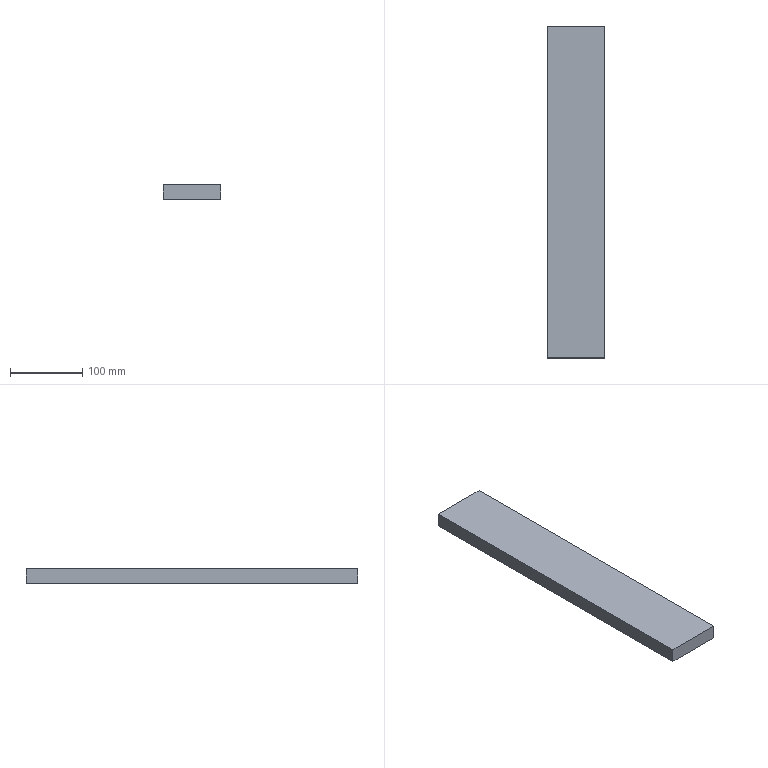Part | SolidWorks | features Extrusion 1 | 1 solid | 6 faces | box 80 x 460 x 20 mm | volume 736000 mm3 | plane 6
STEP:
#1=CARTESIAN_POINT('',(-40.,230.,0.));
#2=VERTEX_POINT('',#1);
#3=CARTESIAN_POINT('',(-40.,-230.,0.));
#4=VERTEX_POINT('',#3);
#5=CARTESIAN_POINT('',(-40.,-230.,0.));
#6=DIRECTION('',(0.,-1.,0.));
#7=VECTOR('',#6,1000.);
#8=LINE('',#5,#7);
#9=EDGE_CURVE('',#2,#4,#8,.T.);
#10=ORIENTED_EDGE('',*,*,#9,.T.);
#11=CARTESIAN_POINT('',(-40.,-230.,20.));
#12=VERTEX_POINT('',#11);
#13=CARTESIAN_POINT('',(-40.,-230.,20.));
#14=DIRECTION('',(0.,0.,-1.));
#15=VECTOR('',#14,1000.);
#16=LINE('',#13,#15);
#17=EDGE_CURVE('',#12,#4,#16,.T.);
#18=ORIENTED_EDGE('',*,*,#17,.F.);
#19=CARTESIAN_POINT('',(-40.,230.,20.));
#20=VERTEX_POINT('',#19);
#21=CARTESIAN_POINT('',(-40.,-230.,20.));
#22=DIRECTION('',(0.,-1.,0.));
#23=VECTOR('',#22,1000.);
#24=LINE('',#21,#23);
#25=EDGE_CURVE('',#20,#12,#24,.T.);
#26=ORIENTED_EDGE('',*,*,#25,.F.);
#27=CARTESIAN_POINT('',(-40.,230.,20.));
#28=DIRECTION('',(0.,0.,-1.));
#29=VECTOR('',#28,1000.);
#30=LINE('',#27,#29);
#31=EDGE_CURVE('',#20,#2,#30,.T.);
#32=ORIENTED_EDGE('',*,*,#31,.T.);
#33=EDGE_LOOP('',(#10,#18,#26,#32));
#34=FACE_OUTER_BOUND('',#33,.T.);
#35=CARTESIAN_POINT('',(-40.,-230.,20.));
#36=DIRECTION('',(1.,0.,0.));
#37=DIRECTION('',(0.,0.,-1.));
#38=AXIS2_PLACEMENT_3D('',#35,#36,#37);
#39=PLANE('',#38);
#40=ADVANCED_FACE('',(#34),#39,.F.);
#41=CARTESIAN_POINT('',(40.,-230.,0.));
#42=VERTEX_POINT('',#41);
#43=CARTESIAN_POINT('',(40.,-230.,0.));
#44=DIRECTION('',(1.,0.,0.));
#45=VECTOR('',#44,1000.);
#46=LINE('',#43,#45);
#47=EDGE_CURVE('',#4,#42,#46,.T.);
#48=ORIENTED_EDGE('',*,*,#47,.T.);
#49=CARTESIAN_POINT('',(40.,-230.,20.));
#50=VERTEX_POINT('',#49);
#51=CARTESIAN_POINT('',(40.,-230.,20.));
#52=DIRECTION('',(0.,0.,-1.));
#53=VECTOR('',#52,1000.);
#54=LINE('',#51,#53);
#55=EDGE_CURVE('',#50,#42,#54,.T.);
#56=ORIENTED_EDGE('',*,*,#55,.F.);
#57=CARTESIAN_POINT('',(40.,-230.,20.));
#58=DIRECTION('',(1.,0.,0.));
#59=VECTOR('',#58,1000.);
#60=LINE('',#57,#59);
#61=EDGE_CURVE('',#12,#50,#60,.T.);
#62=ORIENTED_EDGE('',*,*,#61,.F.);
#63=ORIENTED_EDGE('',*,*,#17,.T.);
#64=EDGE_LOOP('',(#48,#56,#62,#63));
#65=FACE_OUTER_BOUND('',#64,.T.);
#66=CARTESIAN_POINT('',(40.,-230.,20.));
#67=DIRECTION('',(0.,1.,0.));
#68=DIRECTION('',(-1.,0.,0.));
#69=AXIS2_PLACEMENT_3D('',#66,#67,#68);
#70=PLANE('',#69);
#71=ADVANCED_FACE('',(#65),#70,.F.);
#72=CARTESIAN_POINT('',(40.,230.,0.));
#73=VERTEX_POINT('',#72);
#74=CARTESIAN_POINT('',(40.,-230.,0.));
#75=DIRECTION('',(0.,1.,0.));
#76=VECTOR('',#75,1000.);
#77=LINE('',#74,#76);
#78=EDGE_CURVE('',#42,#73,#77,.T.);
#79=ORIENTED_EDGE('',*,*,#78,.T.);
#80=CARTESIAN_POINT('',(40.,230.,20.));
#81=VERTEX_POINT('',#80);
#82=CARTESIAN_POINT('',(40.,230.,20.));
#83=DIRECTION('',(0.,0.,-1.));
#84=VECTOR('',#83,1000.);
#85=LINE('',#82,#84);
#86=EDGE_CURVE('',#81,#73,#85,.T.);
#87=ORIENTED_EDGE('',*,*,#86,.F.);
#88=CARTESIAN_POINT('',(40.,-230.,20.));
#89=DIRECTION('',(0.,1.,0.));
#90=VECTOR('',#89,1000.);
#91=LINE('',#88,#90);
#92=EDGE_CURVE('',#50,#81,#91,.T.);
#93=ORIENTED_EDGE('',*,*,#92,.F.);
#94=ORIENTED_EDGE('',*,*,#55,.T.);
#95=EDGE_LOOP('',(#79,#87,#93,#94));
#96=FACE_OUTER_BOUND('',#95,.T.);
#97=CARTESIAN_POINT('',(40.,-230.,20.));
#98=DIRECTION('',(-1.,0.,0.));
#99=DIRECTION('',(0.,0.,1.));
#100=AXIS2_PLACEMENT_3D('',#97,#98,#99);
#101=PLANE('',#100);
#102=ADVANCED_FACE('',(#96),#101,.F.);
#103=CARTESIAN_POINT('',(40.,230.,0.));
#104=DIRECTION('',(-1.,0.,0.));
#105=VECTOR('',#104,1000.);
#106=LINE('',#103,#105);
#107=EDGE_CURVE('',#73,#2,#106,.T.);
#108=ORIENTED_EDGE('',*,*,#107,.T.);
#109=ORIENTED_EDGE('',*,*,#31,.F.);
#110=CARTESIAN_POINT('',(40.,230.,20.));
#111=DIRECTION('',(-1.,0.,0.));
#112=VECTOR('',#111,1000.);
#113=LINE('',#110,#112);
#114=EDGE_CURVE('',#81,#20,#113,.T.);
#115=ORIENTED_EDGE('',*,*,#114,.F.);
#116=ORIENTED_EDGE('',*,*,#86,.T.);
#117=EDGE_LOOP('',(#108,#109,#115,#116));
#118=FACE_OUTER_BOUND('',#117,.T.);
#119=CARTESIAN_POINT('',(40.,230.,20.));
#120=DIRECTION('',(0.,-1.,0.));
#121=DIRECTION('',(0.,0.,-1.));
#122=AXIS2_PLACEMENT_3D('',#119,#120,#121);
#123=PLANE('',#122);
#124=ADVANCED_FACE('',(#118),#123,.F.);
#125=ORIENTED_EDGE('',*,*,#25,.T.);
#126=ORIENTED_EDGE('',*,*,#61,.T.);
#127=ORIENTED_EDGE('',*,*,#92,.T.);
#128=ORIENTED_EDGE('',*,*,#114,.T.);
#129=EDGE_LOOP('',(#125,#126,#127,#128));
#130=FACE_OUTER_BOUND('',#129,.T.);
#131=CARTESIAN_POINT('',(0.,0.,20.));
#132=DIRECTION('',(0.,0.,1.));
#133=DIRECTION('',(1.,0.,0.));
#134=AXIS2_PLACEMENT_3D('',#131,#132,#133);
#135=PLANE('',#134);
#136=ADVANCED_FACE('',(#130),#135,.T.);
#137=ORIENTED_EDGE('',*,*,#9,.F.);
#138=ORIENTED_EDGE('',*,*,#107,.F.);
#139=ORIENTED_EDGE('',*,*,#78,.F.);
#140=ORIENTED_EDGE('',*,*,#47,.F.);
#141=EDGE_LOOP('',(#137,#138,#139,#140));
#142=FACE_OUTER_BOUND('',#141,.T.);
#143=CARTESIAN_POINT('',(0.,0.,0.));
#144=DIRECTION('',(0.,0.,1.));
#145=DIRECTION('',(1.,0.,0.));
#146=AXIS2_PLACEMENT_3D('',#143,#144,#145);
#147=PLANE('',#146);
#148=ADVANCED_FACE('',(#142),#147,.F.);
#149=CLOSED_SHELL('',(#40,#71,#102,#124,#136,#148));
#150=MANIFOLD_SOLID_BREP('',#149);
#151=CARTESIAN_POINT('',(0.,0.,0.));
#152=DIRECTION('',(0.,0.,1.));
#153=DIRECTION('',(1.,0.,0.));
#154=AXIS2_PLACEMENT_3D('',#151,#152,#153);
#155=(LENGTH_UNIT()NAMED_UNIT(*)SI_UNIT(.MILLI.,.METRE.));
#156=UNCERTAINTY_MEASURE_WITH_UNIT(LENGTH_MEASURE(0.00001),#155,'','');
#157=(NAMED_UNIT(*)PLANE_ANGLE_UNIT()SI_UNIT($,.RADIAN.));
#158=(NAMED_UNIT(*)SI_UNIT($,.STERADIAN.)SOLID_ANGLE_UNIT());
#159=(GEOMETRIC_REPRESENTATION_CONTEXT(3)GLOBAL_UNCERTAINTY_ASSIGNED_CONTEXT((#156))GLOBAL_UNIT_ASSIGNED_CONTEXT((#155,#157,#158))REPRESENTATION_CONTEXT('',''));
#160=ADVANCED_BREP_SHAPE_REPRESENTATION('',(#150,#154),#159);